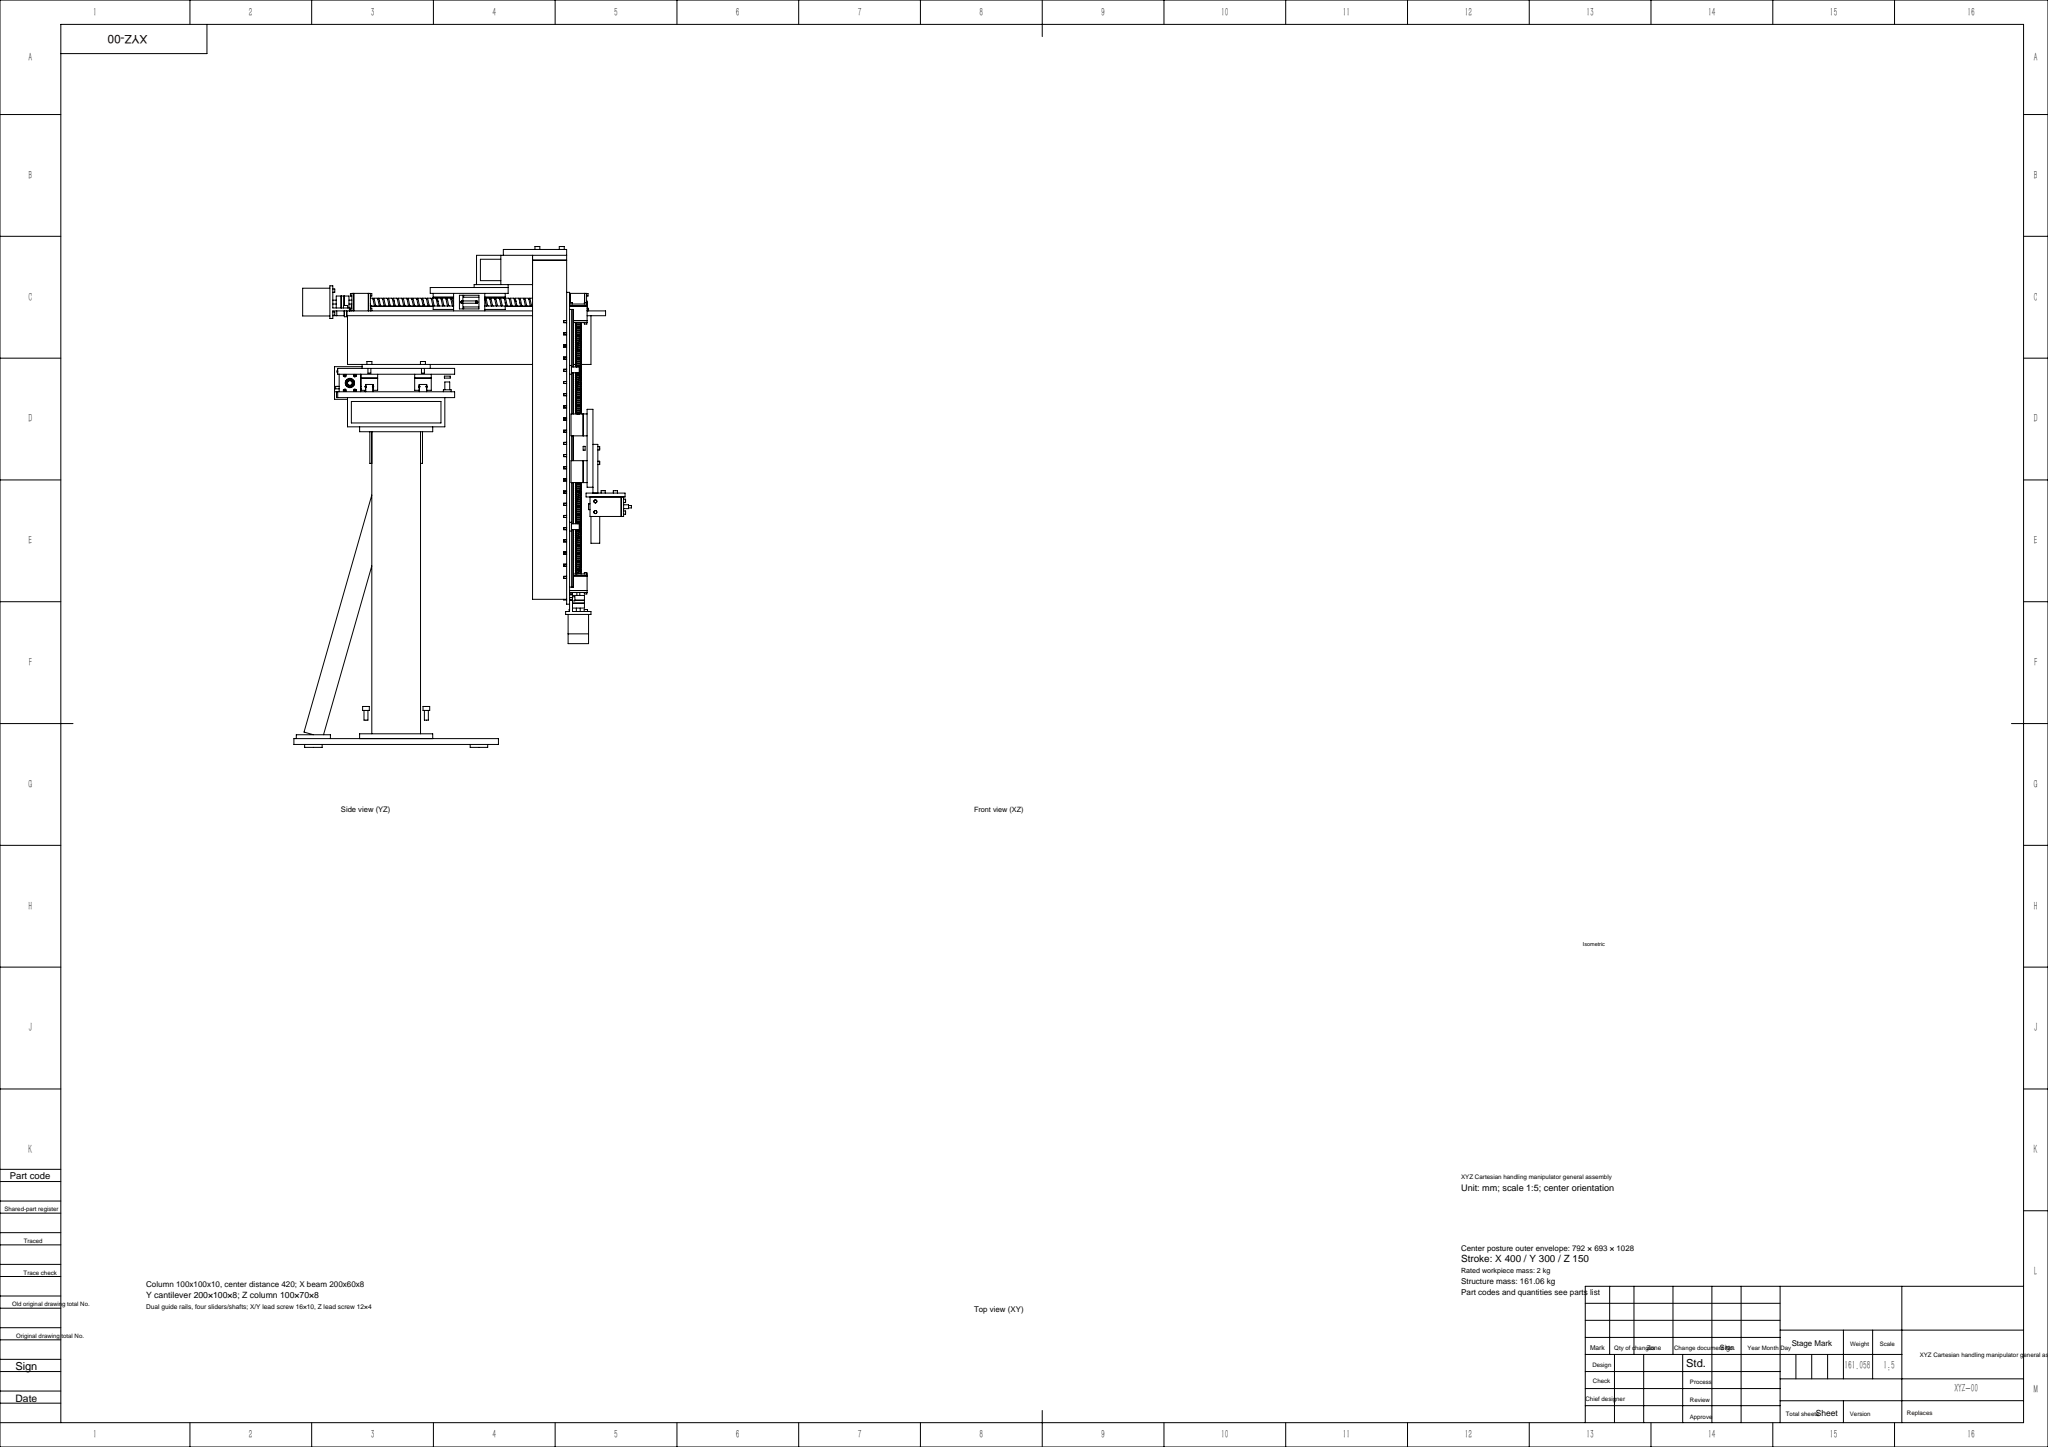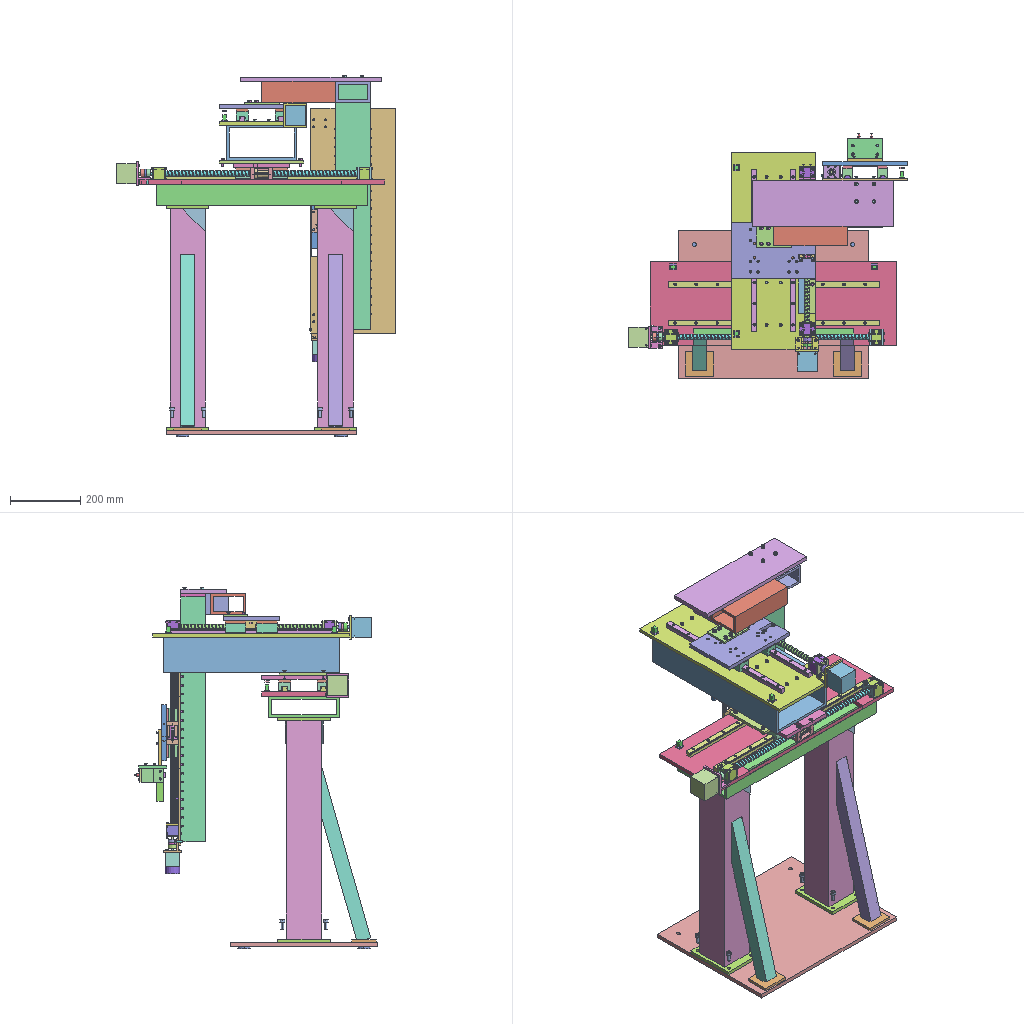Assembly | SolidWorks | 117 different items | 839 placed | box 792 x 693 x 1028 mm
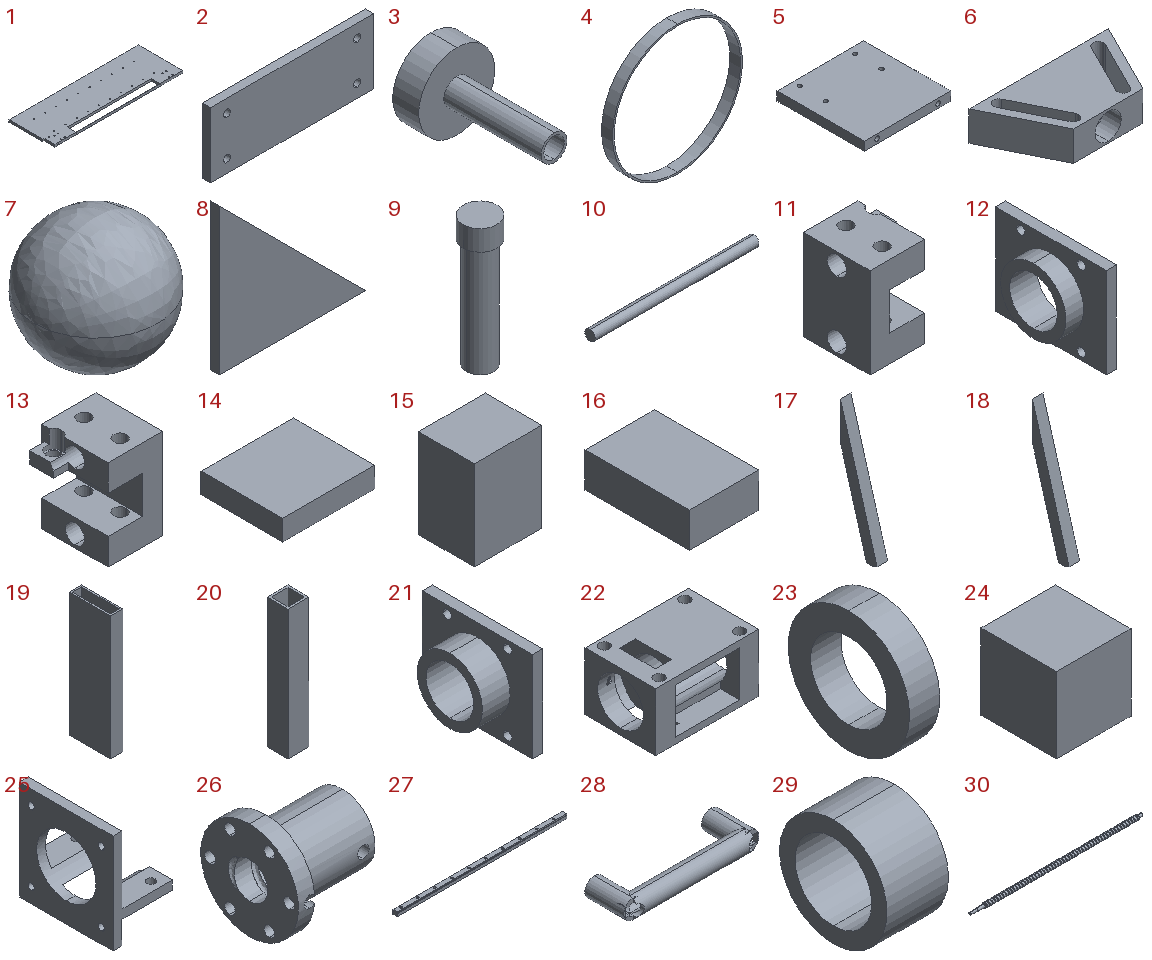Parts list (item | quantity | size | volume | features):
1 | x1 | 700 x 240 x 12 mm | 1744066 mm3 | features BaseBody 1
2 | x1 | 100 x 5 x 40 mm | 19710 mm3 | features BaseBody 1
3 | x1 | 23.4 x 38 x 23.4 mm | 4730 mm3 | features BaseBody 1
4 | x1 | 24 x 2 x 24 mm | 44.673 mm3 | features BaseBody 1
5 | x1 | 100 x 100 x 10 mm | 98969 mm3 | features BaseBody 1
6 | x1 | 56 x 28 x 12 mm | 9686 mm3 | features BaseBody 1
7 | x192 | - | 6.37 mm3 | features BaseBody 1
8 | x4 | 65 x 4 x 65 mm | 8450 mm3 | features BaseBody 1
9 | x2 | 5 x 5 x 19 mm | 259.967 mm3 | features BaseBody 1
10 | x2 | 96 x 6 x 6 mm | 2714 mm3 | features BaseBody 1
11 | x1 | 23 x 22 x 30 mm | 7166 mm3 | features BaseBody 1
12 | x2 | 11 x 44 x 36 mm | 6797 mm3 | features BaseBody 1
13 | x1 | 23 x 22 x 30 mm | 7166 mm3 | features BaseBody 1
14 | x6 | 18 x 16 x 4 mm | 1152 mm3 | features BaseBody 1
15 | x6 | 12 x 10 x 16 mm | 1920 mm3 | features BaseBody 1
16 | x3 | 8 x 12 x 4 mm | 384 mm3 | features BaseBody 1
17 | x1 | 40 x 139.228 x 491.982 mm | 250092 mm3 | features BaseBody 1
18 | x1 | 40 x 139.228 x 491.982 mm | 250092 mm3 | features BaseBody 1
19 | x1 | 60 x 200 x 600 mm | 2342400 mm3 | features BaseBody 1
20 | x2 | 100 x 100 x 620 mm | 2232000 mm3 | features BaseBody 1
21 | x2 | 15 x 44 x 36 mm | 7786 mm3 | features BaseBody 1
22 | x1 | 64 x 44 x 36 mm | 41217 mm3 | features BaseBody 1
23 | x1 | 4 x 16 x 16 mm | 483.774 mm3 | features BaseBody 1
24 | x1 | 80 x 57 x 57 mm | 184911 mm3 | features BaseBody 1
25 | x1 | 40 x 63 x 67 mm | 24720 mm3 | features BaseBody 1
26 | x1 | 40 x 42 x 42 mm | 20795 mm3 | features BaseBody 1
27 | x2 | 600 x 15 x 15 mm | 128298 mm3 | features BaseBody 1
28 | x1 | 34.8 x 11.4 x 4.8 mm | 496.257 mm3 | features BaseBody 1
29 | x3 | 8 x 14 x 14 mm | 603.186 mm3 | features BaseBody 1
30 | x1 | 626 x 16 x 16 mm | 109348 mm3 | features BaseBody 1
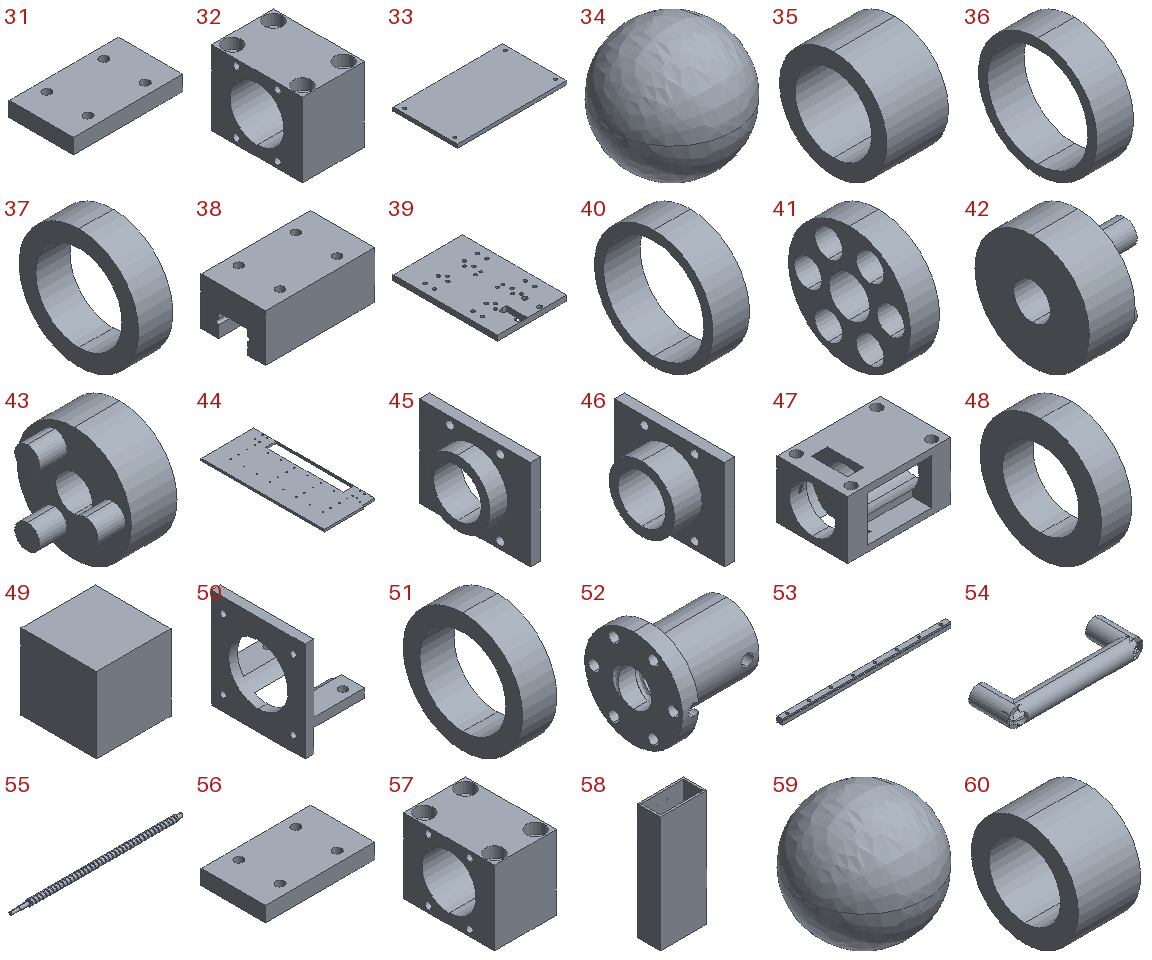31 | x4 | 58 x 34 x 8 mm | 15267 mm3 | features BaseBody 1
32 | x2 | 30 x 44 x 36 mm | 26457 mm3 | features BaseBody 1
33 | x1 | 240 x 140 x 8 mm | 267802 mm3 | features BaseBody 1
34 | x27 | - | 28.73 mm3 | features BaseBody 1
35 | x3 | 8 x 14 x 14 mm | 603.186 mm3 | features BaseBody 1
36 | x3 | 8 x 26 x 26 mm | 1206 mm3 | features BaseBody 1
37 | x2 | 4 x 14 x 14 mm | 295.278 mm3 | features BaseBody 1
38 | x4 | 58 x 34 x 25 mm | 37485 mm3 | features BaseBody 1
39 | x1 | 160 x 240 x 12 mm | 443434 mm3 | features BaseBody 1
40 | x3 | 8 x 26 x 26 mm | 1206 mm3 | features BaseBody 1
41 | x1 | 6 x 25 x 25 mm | 1694 mm3 | features BaseBody 1
42 | x1 | 16 x 25 x 25 mm | 4818 mm3 | features BaseBody 1
43 | x1 | 16 x 25 x 25 mm | 4818 mm3 | features BaseBody 1
44 | x1 | 240 x 560 x 10 mm | 1164432 mm3 | features BaseBody 1
45 | x2 | 11 x 44 x 36 mm | 6797 mm3 | features BaseBody 1
46 | x2 | 15 x 44 x 36 mm | 7786 mm3 | features BaseBody 1
47 | x1 | 64 x 44 x 36 mm | 41217 mm3 | features BaseBody 1
48 | x1 | 4 x 16 x 16 mm | 483.774 mm3 | features BaseBody 1
49 | x1 | 80 x 57 x 57 mm | 184911 mm3 | features BaseBody 1
50 | x1 | 40 x 63 x 67 mm | 24720 mm3 | features BaseBody 1
51 | x2 | 4 x 14 x 14 mm | 295.278 mm3 | features BaseBody 1
52 | x1 | 40 x 42 x 42 mm | 20795 mm3 | features BaseBody 1
53 | x2 | 460 x 15 x 15 mm | 98244 mm3 | features BaseBody 1
54 | x1 | 34.8 x 11.4 x 4.8 mm | 496.257 mm3 | features BaseBody 1
55 | x1 | 486 x 16 x 16 mm | 83136 mm3 | features BaseBody 1
56 | x4 | 58 x 34 x 8 mm | 15267 mm3 | features BaseBody 1
57 | x2 | 30 x 44 x 36 mm | 26457 mm3 | features BaseBody 1
58 | x1 | 200 x 100 x 500 mm | 2270906 mm3 | features BaseBody 1
59 | x27 | - | 11.494 mm3 | features BaseBody 1
60 | x3 | 7 x 12 x 12 mm | 439.823 mm3 | features BaseBody 1
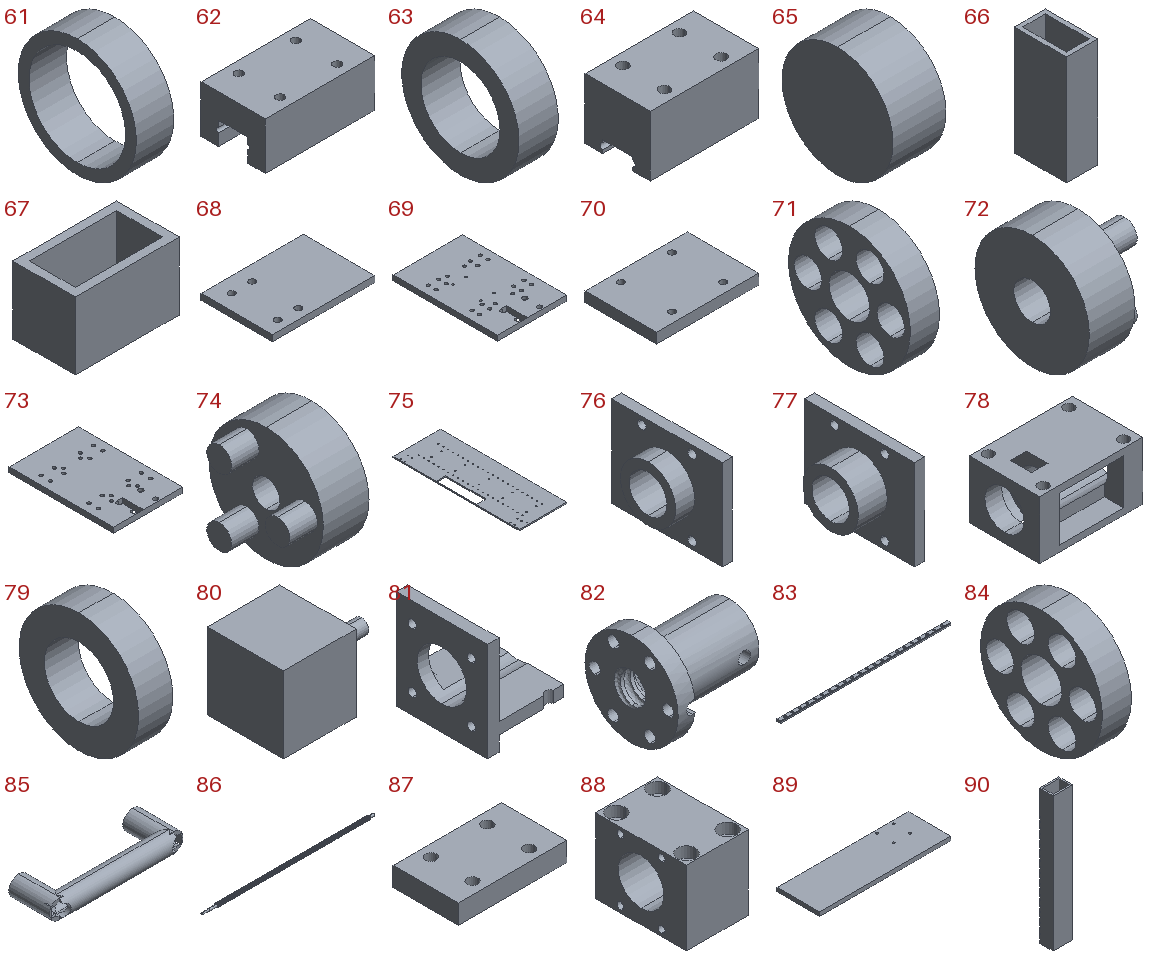61 | x3 | 7 x 22 x 22 mm | 879.646 mm3 | features BaseBody 1
62 | x4 | 58 x 34 x 25 mm | 37485 mm3 | features BaseBody 1
63 | x2 | 4 x 12 x 12 mm | 246.269 mm3 | features BaseBody 1
64 | x4 | 45 x 27 x 25 mm | 26500 mm3 | features BaseBody 1
65 | x1 | 20 x 42 x 42 mm | 27709 mm3 | features BaseBody 1
66 | x1 | 60 x 100 x 210 mm | 483840 mm3 | features BaseBody 1
67 | x1 | 100 x 60 x 65 mm | 149760 mm3 | features BaseBody 1
68 | x1 | 100 x 70 x 6 mm | 41252 mm3 | features BaseBody 1
69 | x1 | 160 x 240 x 12 mm | 444338 mm3 | features BaseBody 1
70 | x1 | 100 x 70 x 10 mm | 68978 mm3 | features BaseBody 1
71 | x1 | 6 x 25 x 25 mm | 1694 mm3 | features BaseBody 1
72 | x1 | 16 x 25 x 25 mm | 4818 mm3 | features BaseBody 1
73 | x1 | 160 x 240 x 12 mm | 444930 mm3 | features BaseBody 1
74 | x1 | 16 x 25 x 25 mm | 5038 mm3 | features BaseBody 1
75 | x1 | 240 x 640 x 6 mm | 856433 mm3 | features BaseBody 1
76 | x2 | 11.5 x 44 x 36 mm | 7018 mm3 | features BaseBody 1
77 | x2 | 15.5 x 44 x 36 mm | 7832 mm3 | features BaseBody 1
78 | x1 | 64 x 44 x 36 mm | 50225 mm3 | features BaseBody 1
79 | x1 | 4 x 14 x 14 mm | 409.632 mm3 | features BaseBody 1
80 | x1 | 64 x 42 x 42 mm | 72019 mm3 | features BaseBody 1
81 | x1 | 40 x 48 x 52 mm | 20561 mm3 | features BaseBody 1
82 | x1 | 40 x 38 x 38 mm | 16524 mm3 | features BaseBody 1
83 | x2 | 570 x 12 x 8 mm | 46406 mm3 | features BaseBody 1
84 | x1 | 6 x 25 x 25 mm | 1694 mm3 | features BaseBody 1
85 | x1 | 32.8 x 11.4 x 4.8 mm | 474.136 mm3 | features BaseBody 1
86 | x1 | 596 x 12 x 12 mm | 49548 mm3 | features BaseBody 1
87 | x4 | 45 x 27 x 8 mm | 9211 mm3 | features BaseBody 1
88 | x2 | 30 x 44 x 36 mm | 31000 mm3 | features BaseBody 1
89 | x1 | 400 x 130 x 12 mm | 622504 mm3 | features BaseBody 1
90 | x1 | 100 x 70 x 696 mm | 1711198 mm3 | features BaseBody 1
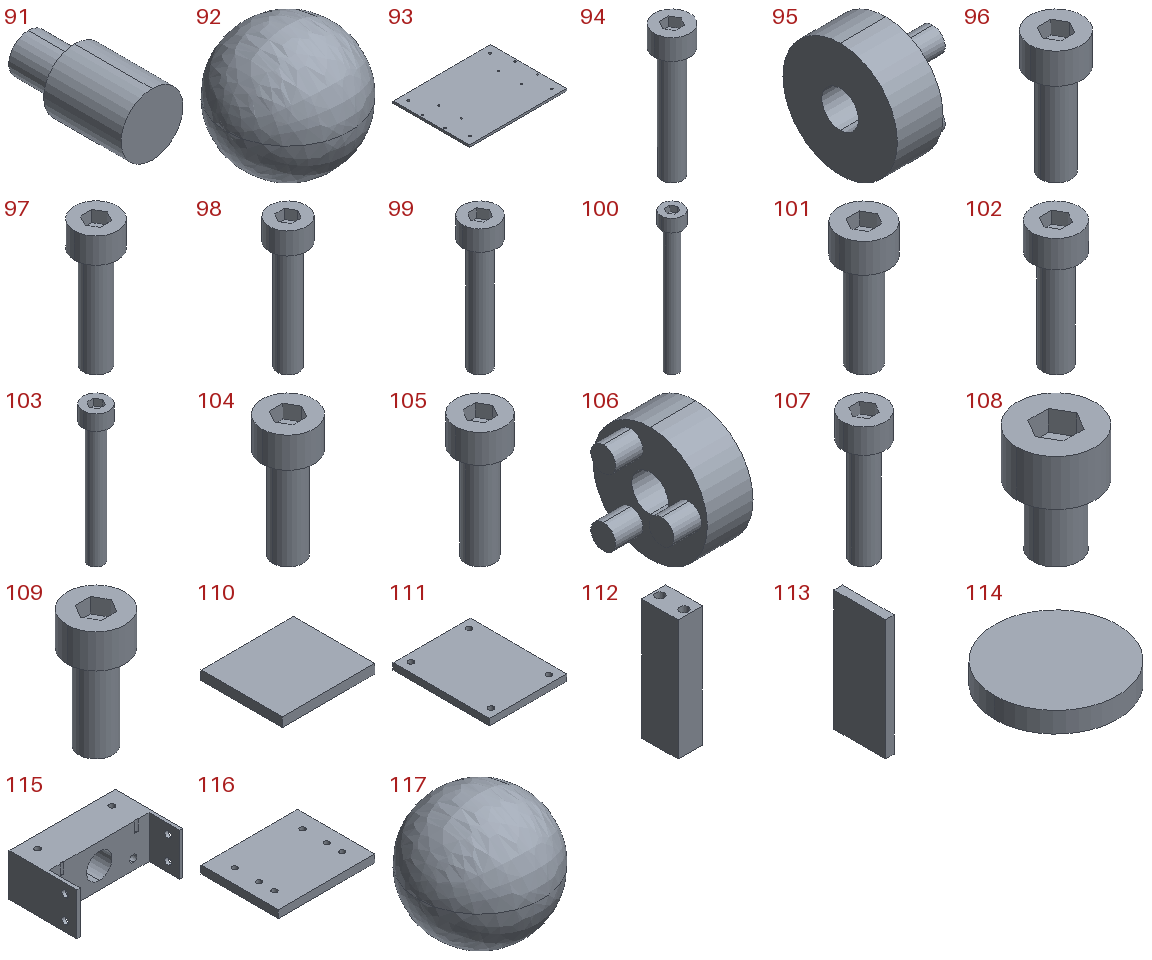91 | x2 | 8 x 16 x 8 mm | 620.465 mm3 | features BaseBody 1
92 | x108 | - | 6.37 mm3 | features BaseBody 1
93 | x1 | 540 x 420 x 12 mm | 2711591 mm3 | features BaseBody 1
94 | x48 | 5.1 x 5.1 x 19 mm | 167.99 mm3 | features BaseBody 1
95 | x1 | 16 x 25 x 25 mm | 4818 mm3 | features BaseBody 1
96 | x16 | 6.8 x 6.8 x 16 mm | 280.912 mm3 | features BaseBody 1
97 | x80 | 6.8 x 6.8 x 20 mm | 331.177 mm3 | features BaseBody 1
98 | x4 | 6.8 x 6.8 x 24 mm | 381.443 mm3 | features BaseBody 1
99 | x48 | 6.8 x 6.8 x 26 mm | 406.575 mm3 | features BaseBody 1
100 | x4 | 6.8 x 6.8 x 44 mm | 632.77 mm3 | features BaseBody 1
101 | x18 | 8.5 x 8.5 x 21 mm | 568.291 mm3 | features BaseBody 1
102 | x12 | 8.5 x 8.5 x 23 mm | 607.561 mm3 | features BaseBody 1
103 | x24 | 8.5 x 8.5 x 45 mm | 1040 mm3 | features BaseBody 1
104 | x8 | 10.2 x 10.2 x 24 mm | 948.077 mm3 | features BaseBody 1
105 | x4 | 10.2 x 10.2 x 26 mm | 1005 mm3 | features BaseBody 1
106 | x1 | 16 x 25 x 25 mm | 4818 mm3 | features BaseBody 1
107 | x12 | 10.2 x 10.2 x 31 mm | 1146 mm3 | features BaseBody 1
108 | x1 | 10.2 x 10.2 x 14 mm | 665.334 mm3 | features BaseBody 1
109 | x8 | 13.6 x 13.6 x 28 mm | 2046 mm3 | features BaseBody 1
110 | x2 | 80 x 70 x 8 mm | 44800 mm3 | features BaseBody 1
111 | x4 | 120 x 150 x 10 mm | 177730 mm3 | features BaseBody 1
112 | x2 | 12 x 18 x 60 mm | 12664 mm3 | features BaseBody 1
113 | x2 | 3 x 18 x 42 mm | 2268 mm3 | features BaseBody 1
114 | x4 | 36 x 36 x 6 mm | 6107 mm3 | features BaseBody 1
115 | x1 | 100 x 64 x 40 mm | 128362 mm3 | features BaseBody 1
116 | x1 | 100 x 80 x 8 mm | 62941 mm3 | features BaseBody 1
117 | x27 | - | 28.73 mm3 | features BaseBody 1